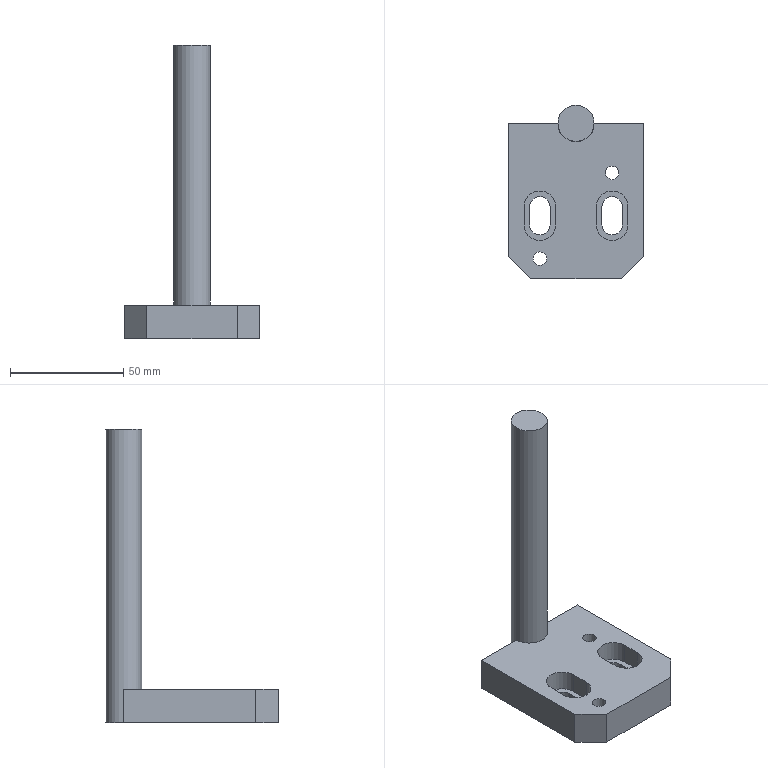Part | NX | features solid 2 | 1 solid | 31 faces | box 60 x 76.5 x 130 mm | volume 77518 mm3 | plane 20 | cylinder 11 | commonest cylinder face diameters 9 x4 14 x4 6 x2 16 x1
STEP:
#1=CARTESIAN_POINT('',(538.,-419.5,-140.));
#2=VERTEX_POINT('',#1);
#3=CARTESIAN_POINT('',(538.,-419.5,-125.));
#4=VERTEX_POINT('',#3);
#5=CARTESIAN_POINT('',(538.,-419.5,-140.));
#6=DIRECTION('',(0.,0.,1.));
#7=VECTOR('',#6,1000.);
#8=LINE('',#5,#7);
#9=EDGE_CURVE('',#2,#4,#8,.T.);
#10=ORIENTED_EDGE('',*,*,#9,.F.);
#11=CARTESIAN_POINT('',(522.,-419.5,-140.));
#12=VERTEX_POINT('',#11);
#13=CARTESIAN_POINT('',(530.,-419.5,-140.));
#14=DIRECTION('',(0.,0.,1.));
#15=DIRECTION('',(1.,0.,0.));
#16=AXIS2_PLACEMENT_3D('',#13,#14,#15);
#17=CIRCLE('',#16,8.);
#18=EDGE_CURVE('',#2,#12,#17,.T.);
#19=ORIENTED_EDGE('',*,*,#18,.T.);
#20=CARTESIAN_POINT('',(522.,-419.5,-125.));
#21=VERTEX_POINT('',#20);
#22=CARTESIAN_POINT('',(522.,-419.5,-140.));
#23=DIRECTION('',(0.,0.,1.));
#24=VECTOR('',#23,1000.);
#25=LINE('',#22,#24);
#26=EDGE_CURVE('',#21,#12,#25,.F.);
#27=ORIENTED_EDGE('',*,*,#26,.F.);
#28=CARTESIAN_POINT('',(530.,-419.5,-125.));
#29=DIRECTION('',(0.,0.,1.));
#30=DIRECTION('',(0.,1.,0.));
#31=AXIS2_PLACEMENT_3D('',#28,#29,#30);
#32=CIRCLE('',#31,8.);
#33=EDGE_CURVE('',#21,#4,#32,.T.);
#34=ORIENTED_EDGE('',*,*,#33,.T.);
#35=EDGE_LOOP('',(#10,#19,#27,#34));
#36=FACE_BOUND('',#35,.T.);
#37=CARTESIAN_POINT('',(522.,-419.5,-10.));
#38=VERTEX_POINT('',#37);
#39=CARTESIAN_POINT('',(530.,-419.5,-10.));
#40=DIRECTION('',(0.,0.,-1.));
#41=DIRECTION('',(-1.,0.,0.));
#42=AXIS2_PLACEMENT_3D('',#39,#40,#41);
#43=CIRCLE('',#42,8.);
#44=EDGE_CURVE('',#38,#38,#43,.F.);
#45=ORIENTED_EDGE('',*,*,#44,.F.);
#46=EDGE_LOOP('',(#45));
#47=FACE_BOUND('',#46,.T.);
#48=CARTESIAN_POINT('',(530.,-419.5,-140.));
#49=DIRECTION('',(0.,0.,1.));
#50=DIRECTION('',(0.,1.,0.));
#51=AXIS2_PLACEMENT_3D('',#48,#49,#50);
#52=CYLINDRICAL_SURFACE('',#51,8.);
#53=ADVANCED_FACE('',(#36,#47),#52,.T.);
#54=ORIENTED_EDGE('',*,*,#44,.T.);
#55=EDGE_LOOP('',(#54));
#56=FACE_BOUND('',#55,.T.);
#57=CARTESIAN_POINT('',(530.,-425.,-10.));
#58=DIRECTION('',(0.,0.,1.));
#59=DIRECTION('',(0.,1.,0.));
#60=AXIS2_PLACEMENT_3D('',#57,#58,#59);
#61=PLANE('',#60);
#62=ADVANCED_FACE('',(#56),#61,.T.);
#63=CARTESIAN_POINT('',(546.,-438.2,-125.));
#64=VERTEX_POINT('',#63);
#65=CARTESIAN_POINT('',(546.,-441.2,-125.));
#66=DIRECTION('',(0.,0.,1.));
#67=DIRECTION('',(0.,1.,0.));
#68=AXIS2_PLACEMENT_3D('',#65,#66,#67);
#69=CIRCLE('',#68,3.);
#70=EDGE_CURVE('',#64,#64,#69,.F.);
#71=ORIENTED_EDGE('',*,*,#70,.T.);
#72=EDGE_LOOP('',(#71));
#73=FACE_BOUND('',#72,.T.);
#74=CARTESIAN_POINT('',(539.,-456.2,-125.));
#75=VERTEX_POINT('',#74);
#76=CARTESIAN_POINT('',(553.,-456.2,-125.));
#77=VERTEX_POINT('',#76);
#78=CARTESIAN_POINT('',(546.,-456.2,-125.));
#79=DIRECTION('',(0.,0.,1.));
#80=DIRECTION('',(0.,1.,0.));
#81=AXIS2_PLACEMENT_3D('',#78,#79,#80);
#82=CIRCLE('',#81,7.);
#83=EDGE_CURVE('',#75,#77,#82,.F.);
#84=ORIENTED_EDGE('',*,*,#83,.T.);
#85=CARTESIAN_POINT('',(553.,-464.2,-125.));
#86=VERTEX_POINT('',#85);
#87=CARTESIAN_POINT('',(553.,-511.,-125.));
#88=DIRECTION('',(0.,-1.,0.));
#89=VECTOR('',#88,1000.);
#90=LINE('',#87,#89);
#91=EDGE_CURVE('',#77,#86,#90,.T.);
#92=ORIENTED_EDGE('',*,*,#91,.T.);
#93=CARTESIAN_POINT('',(539.,-464.2,-125.));
#94=VERTEX_POINT('',#93);
#95=CARTESIAN_POINT('',(546.,-464.2,-125.));
#96=DIRECTION('',(0.,0.,1.));
#97=DIRECTION('',(0.,1.,0.));
#98=AXIS2_PLACEMENT_3D('',#95,#96,#97);
#99=CIRCLE('',#98,7.);
#100=EDGE_CURVE('',#86,#94,#99,.F.);
#101=ORIENTED_EDGE('',*,*,#100,.T.);
#102=CARTESIAN_POINT('',(539.,-511.,-125.));
#103=DIRECTION('',(0.,-1.,0.));
#104=VECTOR('',#103,1000.);
#105=LINE('',#102,#104);
#106=EDGE_CURVE('',#75,#94,#105,.T.);
#107=ORIENTED_EDGE('',*,*,#106,.F.);
#108=EDGE_LOOP('',(#84,#92,#101,#107));
#109=FACE_BOUND('',#108,.T.);
#110=CARTESIAN_POINT('',(514.,-476.2,-125.));
#111=VERTEX_POINT('',#110);
#112=CARTESIAN_POINT('',(514.,-479.2,-125.));
#113=DIRECTION('',(0.,0.,1.));
#114=DIRECTION('',(0.,1.,0.));
#115=AXIS2_PLACEMENT_3D('',#112,#113,#114);
#116=CIRCLE('',#115,3.);
#117=EDGE_CURVE('',#111,#111,#116,.F.);
#118=ORIENTED_EDGE('',*,*,#117,.T.);
#119=EDGE_LOOP('',(#118));
#120=FACE_BOUND('',#119,.T.);
#121=CARTESIAN_POINT('',(507.,-456.2,-125.));
#122=VERTEX_POINT('',#121);
#123=CARTESIAN_POINT('',(507.,-464.2,-125.));
#124=VERTEX_POINT('',#123);
#125=CARTESIAN_POINT('',(507.,-456.2,-125.));
#126=DIRECTION('',(0.,-1.,0.));
#127=VECTOR('',#126,1000.);
#128=LINE('',#125,#127);
#129=EDGE_CURVE('',#122,#124,#128,.T.);
#130=ORIENTED_EDGE('',*,*,#129,.F.);
#131=CARTESIAN_POINT('',(521.,-456.2,-125.));
#132=VERTEX_POINT('',#131);
#133=CARTESIAN_POINT('',(514.,-456.2,-125.));
#134=DIRECTION('',(0.,0.,1.));
#135=DIRECTION('',(0.,1.,0.));
#136=AXIS2_PLACEMENT_3D('',#133,#134,#135);
#137=CIRCLE('',#136,7.);
#138=EDGE_CURVE('',#132,#122,#137,.T.);
#139=ORIENTED_EDGE('',*,*,#138,.F.);
#140=CARTESIAN_POINT('',(521.,-464.2,-125.));
#141=VERTEX_POINT('',#140);
#142=CARTESIAN_POINT('',(521.,-456.2,-125.));
#143=DIRECTION('',(0.,-1.,0.));
#144=VECTOR('',#143,1000.);
#145=LINE('',#142,#144);
#146=EDGE_CURVE('',#132,#141,#145,.T.);
#147=ORIENTED_EDGE('',*,*,#146,.T.);
#148=CARTESIAN_POINT('',(514.,-464.2,-125.));
#149=DIRECTION('',(0.,0.,1.));
#150=DIRECTION('',(0.,1.,0.));
#151=AXIS2_PLACEMENT_3D('',#148,#149,#150);
#152=CIRCLE('',#151,7.);
#153=EDGE_CURVE('',#124,#141,#152,.T.);
#154=ORIENTED_EDGE('',*,*,#153,.F.);
#155=EDGE_LOOP('',(#130,#139,#147,#154));
#156=FACE_BOUND('',#155,.T.);
#157=CARTESIAN_POINT('',(500.,-419.5,-125.));
#158=VERTEX_POINT('',#157);
#159=CARTESIAN_POINT('',(500.,-478.,-125.));
#160=VERTEX_POINT('',#159);
#161=CARTESIAN_POINT('',(500.,-431.,-125.));
#162=DIRECTION('',(0.,-1.,0.));
#163=VECTOR('',#162,1000.);
#164=LINE('',#161,#163);
#165=EDGE_CURVE('',#158,#160,#164,.T.);
#166=ORIENTED_EDGE('',*,*,#165,.T.);
#167=CARTESIAN_POINT('',(510.,-488.,-125.));
#168=VERTEX_POINT('',#167);
#169=CARTESIAN_POINT('',(531.5,-509.5,-125.));
#170=DIRECTION('',(-0.7071,0.7071,0.));
#171=VECTOR('',#170,1000.);
#172=LINE('',#169,#171);
#173=EDGE_CURVE('',#160,#168,#172,.F.);
#174=ORIENTED_EDGE('',*,*,#173,.T.);
#175=CARTESIAN_POINT('',(550.,-488.,-125.));
#176=VERTEX_POINT('',#175);
#177=CARTESIAN_POINT('',(530.,-488.,-125.));
#178=DIRECTION('',(-1.,0.,0.));
#179=VECTOR('',#178,1000.);
#180=LINE('',#177,#179);
#181=EDGE_CURVE('',#168,#176,#180,.F.);
#182=ORIENTED_EDGE('',*,*,#181,.T.);
#183=CARTESIAN_POINT('',(560.,-478.,-125.));
#184=VERTEX_POINT('',#183);
#185=CARTESIAN_POINT('',(528.5,-509.5,-125.));
#186=DIRECTION('',(0.7071,0.7071,0.));
#187=VECTOR('',#186,1000.);
#188=LINE('',#185,#187);
#189=EDGE_CURVE('',#176,#184,#188,.T.);
#190=ORIENTED_EDGE('',*,*,#189,.T.);
#191=CARTESIAN_POINT('',(560.,-419.5,-125.));
#192=VERTEX_POINT('',#191);
#193=CARTESIAN_POINT('',(560.,-431.,-125.));
#194=DIRECTION('',(0.,-1.,0.));
#195=VECTOR('',#194,1000.);
#196=LINE('',#193,#195);
#197=EDGE_CURVE('',#192,#184,#196,.T.);
#198=ORIENTED_EDGE('',*,*,#197,.F.);
#199=CARTESIAN_POINT('',(560.,-419.5,-125.));
#200=DIRECTION('',(-1.,0.,0.));
#201=VECTOR('',#200,1000.);
#202=LINE('',#199,#201);
#203=EDGE_CURVE('',#192,#4,#202,.T.);
#204=ORIENTED_EDGE('',*,*,#203,.T.);
#205=ORIENTED_EDGE('',*,*,#33,.F.);
#206=CARTESIAN_POINT('',(560.,-419.5,-125.));
#207=DIRECTION('',(-1.,0.,0.));
#208=VECTOR('',#207,1000.);
#209=LINE('',#206,#208);
#210=EDGE_CURVE('',#21,#158,#209,.T.);
#211=ORIENTED_EDGE('',*,*,#210,.T.);
#212=EDGE_LOOP('',(#166,#174,#182,#190,#198,#204,#205,#211));
#213=FACE_BOUND('',#212,.T.);
#214=CARTESIAN_POINT('',(530.,-511.,-125.));
#215=DIRECTION('',(0.,0.,1.));
#216=DIRECTION('',(0.,1.,0.));
#217=AXIS2_PLACEMENT_3D('',#214,#215,#216);
#218=PLANE('',#217);
#219=ADVANCED_FACE('',(#73,#109,#120,#156,#213),#218,.T.);
#220=CARTESIAN_POINT('',(546.,-438.2,-140.));
#221=VERTEX_POINT('',#220);
#222=CARTESIAN_POINT('',(546.,-441.2,-140.));
#223=DIRECTION('',(0.,0.,1.));
#224=DIRECTION('',(0.,1.,0.));
#225=AXIS2_PLACEMENT_3D('',#222,#223,#224);
#226=CIRCLE('',#225,3.);
#227=EDGE_CURVE('',#221,#221,#226,.T.);
#228=ORIENTED_EDGE('',*,*,#227,.T.);
#229=EDGE_LOOP('',(#228));
#230=FACE_BOUND('',#229,.T.);
#231=CARTESIAN_POINT('',(509.5,-464.2,-140.));
#232=VERTEX_POINT('',#231);
#233=CARTESIAN_POINT('',(518.5,-464.2,-140.));
#234=VERTEX_POINT('',#233);
#235=CARTESIAN_POINT('',(514.,-464.2,-140.));
#236=DIRECTION('',(0.,0.,1.));
#237=DIRECTION('',(0.,1.,0.));
#238=AXIS2_PLACEMENT_3D('',#235,#236,#237);
#239=CIRCLE('',#238,4.5);
#240=EDGE_CURVE('',#232,#234,#239,.T.);
#241=ORIENTED_EDGE('',*,*,#240,.T.);
#242=CARTESIAN_POINT('',(518.5,-456.2,-140.));
#243=VERTEX_POINT('',#242);
#244=CARTESIAN_POINT('',(518.5,-456.2,-140.));
#245=DIRECTION('',(0.,-1.,0.));
#246=VECTOR('',#245,1000.);
#247=LINE('',#244,#246);
#248=EDGE_CURVE('',#243,#234,#247,.T.);
#249=ORIENTED_EDGE('',*,*,#248,.F.);
#250=CARTESIAN_POINT('',(509.5,-456.2,-140.));
#251=VERTEX_POINT('',#250);
#252=CARTESIAN_POINT('',(514.,-456.2,-140.));
#253=DIRECTION('',(0.,0.,1.));
#254=DIRECTION('',(0.,1.,0.));
#255=AXIS2_PLACEMENT_3D('',#252,#253,#254);
#256=CIRCLE('',#255,4.5);
#257=EDGE_CURVE('',#243,#251,#256,.T.);
#258=ORIENTED_EDGE('',*,*,#257,.T.);
#259=CARTESIAN_POINT('',(509.5,-456.2,-140.));
#260=DIRECTION('',(0.,-1.,0.));
#261=VECTOR('',#260,1000.);
#262=LINE('',#259,#261);
#263=EDGE_CURVE('',#251,#232,#262,.T.);
#264=ORIENTED_EDGE('',*,*,#263,.T.);
#265=EDGE_LOOP('',(#241,#249,#258,#264));
#266=FACE_BOUND('',#265,.T.);
#267=CARTESIAN_POINT('',(514.,-476.2,-140.));
#268=VERTEX_POINT('',#267);
#269=CARTESIAN_POINT('',(514.,-479.2,-140.));
#270=DIRECTION('',(0.,0.,1.));
#271=DIRECTION('',(0.,1.,0.));
#272=AXIS2_PLACEMENT_3D('',#269,#270,#271);
#273=CIRCLE('',#272,3.);
#274=EDGE_CURVE('',#268,#268,#273,.T.);
#275=ORIENTED_EDGE('',*,*,#274,.T.);
#276=EDGE_LOOP('',(#275));
#277=FACE_BOUND('',#276,.T.);
#278=CARTESIAN_POINT('',(541.5,-464.2,-140.));
#279=VERTEX_POINT('',#278);
#280=CARTESIAN_POINT('',(550.5,-464.2,-140.));
#281=VERTEX_POINT('',#280);
#282=CARTESIAN_POINT('',(546.,-464.2,-140.));
#283=DIRECTION('',(0.,0.,1.));
#284=DIRECTION('',(0.,1.,0.));
#285=AXIS2_PLACEMENT_3D('',#282,#283,#284);
#286=CIRCLE('',#285,4.5);
#287=EDGE_CURVE('',#279,#281,#286,.T.);
#288=ORIENTED_EDGE('',*,*,#287,.T.);
#289=CARTESIAN_POINT('',(550.5,-456.2,-140.));
#290=VERTEX_POINT('',#289);
#291=CARTESIAN_POINT('',(550.5,-466.2,-140.));
#292=DIRECTION('',(0.,1.,0.));
#293=VECTOR('',#292,1000.);
#294=LINE('',#291,#293);
#295=EDGE_CURVE('',#281,#290,#294,.T.);
#296=ORIENTED_EDGE('',*,*,#295,.T.);
#297=CARTESIAN_POINT('',(541.5,-456.2,-140.));
#298=VERTEX_POINT('',#297);
#299=CARTESIAN_POINT('',(546.,-456.2,-140.));
#300=DIRECTION('',(0.,0.,1.));
#301=DIRECTION('',(0.,1.,0.));
#302=AXIS2_PLACEMENT_3D('',#299,#300,#301);
#303=CIRCLE('',#302,4.5);
#304=EDGE_CURVE('',#290,#298,#303,.T.);
#305=ORIENTED_EDGE('',*,*,#304,.T.);
#306=CARTESIAN_POINT('',(541.5,-466.2,-140.));
#307=DIRECTION('',(0.,1.,0.));
#308=VECTOR('',#307,1000.);
#309=LINE('',#306,#308);
#310=EDGE_CURVE('',#279,#298,#309,.T.);
#311=ORIENTED_EDGE('',*,*,#310,.F.);
#312=EDGE_LOOP('',(#288,#296,#305,#311));
#313=FACE_BOUND('',#312,.T.);
#314=CARTESIAN_POINT('',(550.,-488.,-140.));
#315=VERTEX_POINT('',#314);
#316=CARTESIAN_POINT('',(510.,-488.,-140.));
#317=VERTEX_POINT('',#316);
#318=CARTESIAN_POINT('',(570.,-488.,-140.));
#319=DIRECTION('',(1.,0.,0.));
#320=VECTOR('',#319,1000.);
#321=LINE('',#318,#320);
#322=EDGE_CURVE('',#315,#317,#321,.F.);
#323=ORIENTED_EDGE('',*,*,#322,.T.);
#324=CARTESIAN_POINT('',(500.,-478.,-140.));
#325=VERTEX_POINT('',#324);
#326=CARTESIAN_POINT('',(510.,-488.,-140.));
#327=DIRECTION('',(0.7071,-0.7071,0.));
#328=VECTOR('',#327,1000.);
#329=LINE('',#326,#328);
#330=EDGE_CURVE('',#317,#325,#329,.F.);
#331=ORIENTED_EDGE('',*,*,#330,.T.);
#332=CARTESIAN_POINT('',(500.,-419.5,-140.));
#333=VERTEX_POINT('',#332);
#334=CARTESIAN_POINT('',(500.,-431.,-140.));
#335=DIRECTION('',(0.,-1.,0.));
#336=VECTOR('',#335,1000.);
#337=LINE('',#334,#336);
#338=EDGE_CURVE('',#333,#325,#337,.T.);
#339=ORIENTED_EDGE('',*,*,#338,.F.);
#340=CARTESIAN_POINT('',(560.,-419.5,-140.));
#341=DIRECTION('',(-1.,0.,0.));
#342=VECTOR('',#341,1000.);
#343=LINE('',#340,#342);
#344=EDGE_CURVE('',#12,#333,#343,.T.);
#345=ORIENTED_EDGE('',*,*,#344,.F.);
#346=ORIENTED_EDGE('',*,*,#18,.F.);
#347=CARTESIAN_POINT('',(560.,-419.5,-140.));
#348=VERTEX_POINT('',#347);
#349=CARTESIAN_POINT('',(560.,-419.5,-140.));
#350=DIRECTION('',(-1.,0.,0.));
#351=VECTOR('',#350,1000.);
#352=LINE('',#349,#351);
#353=EDGE_CURVE('',#348,#2,#352,.T.);
#354=ORIENTED_EDGE('',*,*,#353,.F.);
#355=CARTESIAN_POINT('',(560.,-478.,-140.));
#356=VERTEX_POINT('',#355);
#357=CARTESIAN_POINT('',(560.,-431.,-140.));
#358=DIRECTION('',(0.,-1.,0.));
#359=VECTOR('',#358,1000.);
#360=LINE('',#357,#359);
#361=EDGE_CURVE('',#348,#356,#360,.T.);
#362=ORIENTED_EDGE('',*,*,#361,.T.);
#363=CARTESIAN_POINT('',(560.,-478.,-140.));
#364=DIRECTION('',(-0.7071,-0.7071,0.));
#365=VECTOR('',#364,1000.);
#366=LINE('',#363,#365);
#367=EDGE_CURVE('',#356,#315,#366,.T.);
#368=ORIENTED_EDGE('',*,*,#367,.T.);
#369=EDGE_LOOP('',(#323,#331,#339,#345,#346,#354,#362,#368));
#370=FACE_BOUND('',#369,.T.);
#371=CARTESIAN_POINT('',(530.,-511.,-140.));
#372=DIRECTION('',(0.,0.,1.));
#373=DIRECTION('',(0.,1.,0.));
#374=AXIS2_PLACEMENT_3D('',#371,#372,#373);
#375=PLANE('',#374);
#376=ADVANCED_FACE('',(#230,#266,#277,#313,#370),#375,.F.);
#377=ORIENTED_EDGE('',*,*,#197,.T.);
#378=CARTESIAN_POINT('',(560.,-478.,-125.));
#379=DIRECTION('',(0.,0.,-1.));
#380=VECTOR('',#379,1000.);
#381=LINE('',#378,#380);
#382=EDGE_CURVE('',#184,#356,#381,.T.);
#383=ORIENTED_EDGE('',*,*,#382,.T.);
#384=ORIENTED_EDGE('',*,*,#361,.F.);
#385=CARTESIAN_POINT('',(560.,-419.5,-125.));
#386=DIRECTION('',(0.,0.,-1.));
#387=VECTOR('',#386,1000.);
#388=LINE('',#385,#387);
#389=EDGE_CURVE('',#192,#348,#388,.T.);
#390=ORIENTED_EDGE('',*,*,#389,.F.);
#391=EDGE_LOOP('',(#377,#383,#384,#390));
#392=FACE_BOUND('',#391,.T.);
#393=CARTESIAN_POINT('',(560.,-431.,-125.));
#394=DIRECTION('',(1.,0.,0.));
#395=DIRECTION('',(0.,0.,-1.));
#396=AXIS2_PLACEMENT_3D('',#393,#394,#395);
#397=PLANE('',#396);
#398=ADVANCED_FACE('',(#392),#397,.T.);
#399=ORIENTED_EDGE('',*,*,#338,.T.);
#400=CARTESIAN_POINT('',(500.,-478.,-125.));
#401=DIRECTION('',(0.,0.,1.));
#402=VECTOR('',#401,1000.);
#403=LINE('',#400,#402);
#404=EDGE_CURVE('',#325,#160,#403,.T.);
#405=ORIENTED_EDGE('',*,*,#404,.T.);
#406=ORIENTED_EDGE('',*,*,#165,.F.);
#407=CARTESIAN_POINT('',(500.,-419.5,-125.));
#408=DIRECTION('',(0.,0.,-1.));
#409=VECTOR('',#408,1000.);
#410=LINE('',#407,#409);
#411=EDGE_CURVE('',#158,#333,#410,.T.);
#412=ORIENTED_EDGE('',*,*,#411,.T.);
#413=EDGE_LOOP('',(#399,#405,#406,#412));
#414=FACE_BOUND('',#413,.T.);
#415=CARTESIAN_POINT('',(500.,-431.,-125.));
#416=DIRECTION('',(1.,0.,0.));
#417=DIRECTION('',(0.,1.,0.));
#418=AXIS2_PLACEMENT_3D('',#415,#416,#417);
#419=PLANE('',#418);
#420=ADVANCED_FACE('',(#414),#419,.F.);
#421=ORIENTED_EDGE('',*,*,#353,.T.);
#422=ORIENTED_EDGE('',*,*,#9,.T.);
#423=ORIENTED_EDGE('',*,*,#203,.F.);
#424=ORIENTED_EDGE('',*,*,#389,.T.);
#425=EDGE_LOOP('',(#421,#422,#423,#424));
#426=FACE_BOUND('',#425,.T.);
#427=CARTESIAN_POINT('',(560.,-419.5,-125.));
#428=DIRECTION('',(0.,-1.,0.));
#429=DIRECTION('',(0.,0.,1.));
#430=AXIS2_PLACEMENT_3D('',#427,#428,#429);
#431=PLANE('',#430);
#432=ADVANCED_FACE('',(#426),#431,.F.);
#433=CARTESIAN_POINT('',(518.5,-456.2,-134.));
#434=VERTEX_POINT('',#433);
#435=CARTESIAN_POINT('',(518.5,-464.2,-134.));
#436=VERTEX_POINT('',#435);
#437=CARTESIAN_POINT('',(518.5,-456.2,-134.));
#438=DIRECTION('',(0.,-1.,0.));
#439=VECTOR('',#438,1000.);
#440=LINE('',#437,#439);
#441=EDGE_CURVE('',#434,#436,#440,.T.);
#442=ORIENTED_EDGE('',*,*,#441,.F.);
#443=CARTESIAN_POINT('',(518.5,-456.2,-124.));
#444=DIRECTION('',(0.,0.,-1.));
#445=VECTOR('',#444,1000.);
#446=LINE('',#443,#445);
#447=EDGE_CURVE('',#434,#243,#446,.T.);
#448=ORIENTED_EDGE('',*,*,#447,.T.);
#449=ORIENTED_EDGE('',*,*,#248,.T.);
#450=CARTESIAN_POINT('',(518.5,-464.2,-124.));
#451=DIRECTION('',(0.,0.,-1.));
#452=VECTOR('',#451,1000.);
#453=LINE('',#450,#452);
#454=EDGE_CURVE('',#436,#234,#453,.T.);
#455=ORIENTED_EDGE('',*,*,#454,.F.);
#456=EDGE_LOOP('',(#442,#448,#449,#455));
#457=FACE_BOUND('',#456,.T.);
#458=CARTESIAN_POINT('',(518.5,-456.2,-124.));
#459=DIRECTION('',(1.,0.,0.));
#460=DIRECTION('',(0.,0.,-1.));
#461=AXIS2_PLACEMENT_3D('',#458,#459,#460);
#462=PLANE('',#461);
#463=ADVANCED_FACE('',(#457),#462,.F.);
#464=ORIENTED_EDGE('',*,*,#447,.F.);
#465=CARTESIAN_POINT('',(509.5,-456.2,-134.));
#466=VERTEX_POINT('',#465);
#467=CARTESIAN_POINT('',(514.,-456.2,-134.));
#468=DIRECTION('',(0.,0.,1.));
#469=DIRECTION('',(0.,1.,0.));
#470=AXIS2_PLACEMENT_3D('',#467,#468,#469);
#471=CIRCLE('',#470,4.5);
#472=EDGE_CURVE('',#434,#466,#471,.T.);
#473=ORIENTED_EDGE('',*,*,#472,.T.);
#474=CARTESIAN_POINT('',(509.5,-456.2,-124.));
#475=DIRECTION('',(0.,0.,-1.));
#476=VECTOR('',#475,1000.);
#477=LINE('',#474,#476);
#478=EDGE_CURVE('',#466,#251,#477,.T.);
#479=ORIENTED_EDGE('',*,*,#478,.T.);
#480=ORIENTED_EDGE('',*,*,#257,.F.);
#481=EDGE_LOOP('',(#464,#473,#479,#480));
#482=FACE_BOUND('',#481,.T.);
#483=CARTESIAN_POINT('',(514.,-456.2,-124.));
#484=DIRECTION('',(0.,0.,-1.));
#485=DIRECTION('',(0.,-1.,0.));
#486=AXIS2_PLACEMENT_3D('',#483,#484,#485);
#487=CYLINDRICAL_SURFACE('',#486,4.5);
#488=ADVANCED_FACE('',(#482),#487,.F.);
#489=ORIENTED_EDGE('',*,*,#478,.F.);
#490=CARTESIAN_POINT('',(509.5,-464.2,-134.));
#491=VERTEX_POINT('',#490);
#492=CARTESIAN_POINT('',(509.5,-456.2,-134.));
#493=DIRECTION('',(0.,-1.,0.));
#494=VECTOR('',#493,1000.);
#495=LINE('',#492,#494);
#496=EDGE_CURVE('',#466,#491,#495,.T.);
#497=ORIENTED_EDGE('',*,*,#496,.T.);
#498=CARTESIAN_POINT('',(509.5,-464.2,-124.));
#499=DIRECTION('',(0.,0.,-1.));
#500=VECTOR('',#499,1000.);
#501=LINE('',#498,#500);
#502=EDGE_CURVE('',#491,#232,#501,.T.);
#503=ORIENTED_EDGE('',*,*,#502,.T.);
#504=ORIENTED_EDGE('',*,*,#263,.F.);
#505=EDGE_LOOP('',(#489,#497,#503,#504));
#506=FACE_BOUND('',#505,.T.);
#507=CARTESIAN_POINT('',(509.5,-456.2,-124.));
#508=DIRECTION('',(1.,0.,0.));
#509=DIRECTION('',(0.,0.,-1.));
#510=AXIS2_PLACEMENT_3D('',#507,#508,#509);
#511=PLANE('',#510);
#512=ADVANCED_FACE('',(#506),#511,.T.);
#513=ORIENTED_EDGE('',*,*,#502,.F.);
#514=CARTESIAN_POINT('',(514.,-464.2,-134.));
#515=DIRECTION('',(0.,0.,1.));
#516=DIRECTION('',(0.,1.,0.));
#517=AXIS2_PLACEMENT_3D('',#514,#515,#516);
#518=CIRCLE('',#517,4.5);
#519=EDGE_CURVE('',#491,#436,#518,.T.);
#520=ORIENTED_EDGE('',*,*,#519,.T.);
#521=ORIENTED_EDGE('',*,*,#454,.T.);
#522=ORIENTED_EDGE('',*,*,#240,.F.);
#523=EDGE_LOOP('',(#513,#520,#521,#522));
#524=FACE_BOUND('',#523,.T.);
#525=CARTESIAN_POINT('',(514.,-464.2,-124.));
#526=DIRECTION('',(0.,0.,-1.));
#527=DIRECTION('',(0.,-1.,0.));
#528=AXIS2_PLACEMENT_3D('',#525,#526,#527);
#529=CYLINDRICAL_SURFACE('',#528,4.5);
#530=ADVANCED_FACE('',(#524),#529,.F.);
#531=ORIENTED_EDGE('',*,*,#210,.F.);
#532=ORIENTED_EDGE('',*,*,#26,.T.);
#533=ORIENTED_EDGE('',*,*,#344,.T.);
#534=ORIENTED_EDGE('',*,*,#411,.F.);
#535=EDGE_LOOP('',(#531,#532,#533,#534));
#536=FACE_BOUND('',#535,.T.);
#537=CARTESIAN_POINT('',(560.,-419.5,-125.));
#538=DIRECTION('',(0.,-1.,0.));
#539=DIRECTION('',(0.,0.,1.));
#540=AXIS2_PLACEMENT_3D('',#537,#538,#539);
#541=PLANE('',#540);
#542=ADVANCED_FACE('',(#536),#541,.F.);
#543=CARTESIAN_POINT('',(553.,-456.2,-134.));
#544=VERTEX_POINT('',#543);
#545=CARTESIAN_POINT('',(553.,-456.2,-124.));
#546=DIRECTION('',(0.,0.,-1.));
#547=VECTOR('',#546,1000.);
#548=LINE('',#545,#547);
#549=EDGE_CURVE('',#77,#544,#548,.T.);
#550=ORIENTED_EDGE('',*,*,#549,.T.);
#551=CARTESIAN_POINT('',(553.,-464.2,-134.));
#552=VERTEX_POINT('',#551);
#553=CARTESIAN_POINT('',(553.,-466.2,-134.));
#554=DIRECTION('',(0.,1.,0.));
#555=VECTOR('',#554,1000.);
#556=LINE('',#553,#555);
#557=EDGE_CURVE('',#552,#544,#556,.T.);
#558=ORIENTED_EDGE('',*,*,#557,.F.);
#559=CARTESIAN_POINT('',(553.,-464.2,-124.));
#560=DIRECTION('',(0.,0.,-1.));
#561=VECTOR('',#560,1000.);
#562=LINE('',#559,#561);
#563=EDGE_CURVE('',#86,#552,#562,.T.);
#564=ORIENTED_EDGE('',*,*,#563,.F.);
#565=ORIENTED_EDGE('',*,*,#91,.F.);
#566=EDGE_LOOP('',(#550,#558,#564,#565));
#567=FACE_BOUND('',#566,.T.);
#568=CARTESIAN_POINT('',(553.,-466.2,-124.));
#569=DIRECTION('',(-1.,0.,0.));
#570=DIRECTION('',(0.,0.,1.));
#571=AXIS2_PLACEMENT_3D('',#568,#569,#570);
#572=PLANE('',#571);
#573=ADVANCED_FACE('',(#567),#572,.T.);
#574=CARTESIAN_POINT('',(539.,-456.2,-134.));
#575=VERTEX_POINT('',#574);
#576=CARTESIAN_POINT('',(539.,-456.2,-124.));
#577=DIRECTION('',(0.,0.,-1.));
#578=VECTOR('',#577,1000.);
#579=LINE('',#576,#578);
#580=EDGE_CURVE('',#75,#575,#579,.T.);
#581=ORIENTED_EDGE('',*,*,#580,.T.);
#582=CARTESIAN_POINT('',(546.,-456.2,-134.));
#583=DIRECTION('',(0.,0.,1.));
#584=DIRECTION('',(0.,1.,0.));
#585=AXIS2_PLACEMENT_3D('',#582,#583,#584);
#586=CIRCLE('',#585,7.);
#587=EDGE_CURVE('',#544,#575,#586,.T.);
#588=ORIENTED_EDGE('',*,*,#587,.F.);
#589=ORIENTED_EDGE('',*,*,#549,.F.);
#590=ORIENTED_EDGE('',*,*,#83,.F.);
#591=EDGE_LOOP('',(#581,#588,#589,#590));
#592=FACE_BOUND('',#591,.T.);
#593=CARTESIAN_POINT('',(546.,-456.2,-124.));
#594=DIRECTION('',(0.,0.,-1.));
#595=DIRECTION('',(0.,-1.,0.));
#596=AXIS2_PLACEMENT_3D('',#593,#594,#595);
#597=CYLINDRICAL_SURFACE('',#596,7.);
#598=ADVANCED_FACE('',(#592),#597,.F.);
#599=ORIENTED_EDGE('',*,*,#106,.T.);
#600=CARTESIAN_POINT('',(539.,-464.2,-134.));
#601=VERTEX_POINT('',#600);
#602=CARTESIAN_POINT('',(539.,-464.2,-124.));
#603=DIRECTION('',(0.,0.,-1.));
#604=VECTOR('',#603,1000.);
#605=LINE('',#602,#604);
#606=EDGE_CURVE('',#94,#601,#605,.T.);
#607=ORIENTED_EDGE('',*,*,#606,.T.);
#608=CARTESIAN_POINT('',(539.,-466.2,-134.));
#609=DIRECTION('',(0.,1.,0.));
#610=VECTOR('',#609,1000.);
#611=LINE('',#608,#610);
#612=EDGE_CURVE('',#601,#575,#611,.T.);
#613=ORIENTED_EDGE('',*,*,#612,.T.);
#614=ORIENTED_EDGE('',*,*,#580,.F.);
#615=EDGE_LOOP('',(#599,#607,#613,#614));
#616=FACE_BOUND('',#615,.T.);
#617=CARTESIAN_POINT('',(539.,-466.2,-124.));
#618=DIRECTION('',(-1.,0.,0.));
#619=DIRECTION('',(0.,0.,1.));
#620=AXIS2_PLACEMENT_3D('',#617,#618,#619);
#621=PLANE('',#620);
#622=ADVANCED_FACE('',(#616),#621,.F.);
#623=ORIENTED_EDGE('',*,*,#563,.T.);
#624=CARTESIAN_POINT('',(546.,-464.2,-134.));
#625=DIRECTION('',(0.,0.,1.));
#626=DIRECTION('',(0.,1.,0.));
#627=AXIS2_PLACEMENT_3D('',#624,#625,#626);
#628=CIRCLE('',#627,7.);
#629=EDGE_CURVE('',#601,#552,#628,.T.);
#630=ORIENTED_EDGE('',*,*,#629,.F.);
#631=ORIENTED_EDGE('',*,*,#606,.F.);
#632=ORIENTED_EDGE('',*,*,#100,.F.);
#633=EDGE_LOOP('',(#623,#630,#631,#632));
#634=FACE_BOUND('',#633,.T.);
#635=CARTESIAN_POINT('',(546.,-464.2,-124.));
#636=DIRECTION('',(0.,0.,-1.));
#637=DIRECTION('',(0.,-1.,0.));
#638=AXIS2_PLACEMENT_3D('',#635,#636,#637);
#639=CYLINDRICAL_SURFACE('',#638,7.);
#640=ADVANCED_FACE('',(#634),#639,.F.);
#641=CARTESIAN_POINT('',(550.5,-464.2,-134.));
#642=VERTEX_POINT('',#641);
#643=CARTESIAN_POINT('',(550.5,-456.2,-134.));
#644=VERTEX_POINT('',#643);
#645=CARTESIAN_POINT('',(550.5,-466.2,-134.));
#646=DIRECTION('',(0.,1.,0.));
#647=VECTOR('',#646,1000.);
#648=LINE('',#645,#647);
#649=EDGE_CURVE('',#642,#644,#648,.T.);
#650=ORIENTED_EDGE('',*,*,#649,.F.);
#651=CARTESIAN_POINT('',(541.5,-464.2,-134.));
#652=VERTEX_POINT('',#651);
#653=CARTESIAN_POINT('',(546.,-464.2,-134.));
#654=DIRECTION('',(0.,0.,1.));
#655=DIRECTION('',(0.,1.,0.));
#656=AXIS2_PLACEMENT_3D('',#653,#654,#655);
#657=CIRCLE('',#656,4.5);
#658=EDGE_CURVE('',#652,#642,#657,.T.);
#659=ORIENTED_EDGE('',*,*,#658,.F.);
#660=CARTESIAN_POINT('',(541.5,-456.2,-134.));
#661=VERTEX_POINT('',#660);
#662=CARTESIAN_POINT('',(541.5,-466.2,-134.));
#663=DIRECTION('',(0.,1.,0.));
#664=VECTOR('',#663,1000.);
#665=LINE('',#662,#664);
#666=EDGE_CURVE('',#652,#661,#665,.T.);
#667=ORIENTED_EDGE('',*,*,#666,.T.);
#668=CARTESIAN_POINT('',(546.,-456.2,-134.));
#669=DIRECTION('',(0.,0.,1.));
#670=DIRECTION('',(0.,1.,0.));
#671=AXIS2_PLACEMENT_3D('',#668,#669,#670);
#672=CIRCLE('',#671,4.5);
#673=EDGE_CURVE('',#644,#661,#672,.T.);
#674=ORIENTED_EDGE('',*,*,#673,.F.);
#675=EDGE_LOOP('',(#650,#659,#667,#674));
#676=FACE_BOUND('',#675,.T.);
#677=ORIENTED_EDGE('',*,*,#557,.T.);
#678=ORIENTED_EDGE('',*,*,#587,.T.);
#679=ORIENTED_EDGE('',*,*,#612,.F.);
#680=ORIENTED_EDGE('',*,*,#629,.T.);
#681=EDGE_LOOP('',(#677,#678,#679,#680));
#682=FACE_BOUND('',#681,.T.);
#683=CARTESIAN_POINT('',(546.,-466.2,-134.));
#684=DIRECTION('',(0.,0.,1.));
#685=DIRECTION('',(0.,1.,0.));
#686=AXIS2_PLACEMENT_3D('',#683,#684,#685);
#687=PLANE('',#686);
#688=ADVANCED_FACE('',(#676,#682),#687,.T.);
#689=ORIENTED_EDGE('',*,*,#117,.F.);
#690=EDGE_LOOP('',(#689));
#691=FACE_BOUND('',#690,.T.);
#692=ORIENTED_EDGE('',*,*,#274,.F.);
#693=EDGE_LOOP('',(#692));
#694=FACE_BOUND('',#693,.T.);
#695=CARTESIAN_POINT('',(514.,-479.2,-124.));
#696=DIRECTION('',(0.,0.,-1.));
#697=DIRECTION('',(0.,-1.,0.));
#698=AXIS2_PLACEMENT_3D('',#695,#696,#697);
#699=CYLINDRICAL_SURFACE('',#698,3.);
#700=ADVANCED_FACE('',(#691,#694),#699,.F.);
#701=ORIENTED_EDGE('',*,*,#70,.F.);
#702=EDGE_LOOP('',(#701));
#703=FACE_BOUND('',#702,.T.);
#704=ORIENTED_EDGE('',*,*,#227,.F.);
#705=EDGE_LOOP('',(#704));
#706=FACE_BOUND('',#705,.T.);
#707=CARTESIAN_POINT('',(546.,-441.2,-124.));
#708=DIRECTION('',(0.,0.,-1.));
#709=DIRECTION('',(0.,-1.,0.));
#710=AXIS2_PLACEMENT_3D('',#707,#708,#709);
#711=CYLINDRICAL_SURFACE('',#710,3.);
#712=ADVANCED_FACE('',(#703,#706),#711,.F.);
#713=CARTESIAN_POINT('',(507.,-456.2,-134.));
#714=VERTEX_POINT('',#713);
#715=CARTESIAN_POINT('',(507.,-464.2,-134.));
#716=VERTEX_POINT('',#715);
#717=CARTESIAN_POINT('',(507.,-456.2,-134.));
#718=DIRECTION('',(0.,-1.,0.));
#719=VECTOR('',#718,1000.);
#720=LINE('',#717,#719);
#721=EDGE_CURVE('',#714,#716,#720,.T.);
#722=ORIENTED_EDGE('',*,*,#721,.T.);
#723=CARTESIAN_POINT('',(521.,-464.2,-134.));
#724=VERTEX_POINT('',#723);
#725=CARTESIAN_POINT('',(514.,-464.2,-134.));
#726=DIRECTION('',(0.,0.,1.));
#727=DIRECTION('',(0.,1.,0.));
#728=AXIS2_PLACEMENT_3D('',#725,#726,#727);
#729=CIRCLE('',#728,7.);
#730=EDGE_CURVE('',#716,#724,#729,.T.);
#731=ORIENTED_EDGE('',*,*,#730,.T.);
#732=CARTESIAN_POINT('',(521.,-456.2,-134.));
#733=VERTEX_POINT('',#732);
#734=CARTESIAN_POINT('',(521.,-456.2,-134.));
#735=DIRECTION('',(0.,-1.,0.));
#736=VECTOR('',#735,1000.);
#737=LINE('',#734,#736);
#738=EDGE_CURVE('',#733,#724,#737,.T.);
#739=ORIENTED_EDGE('',*,*,#738,.F.);
#740=CARTESIAN_POINT('',(514.,-456.2,-134.));
#741=DIRECTION('',(0.,0.,1.));
#742=DIRECTION('',(0.,1.,0.));
#743=AXIS2_PLACEMENT_3D('',#740,#741,#742);
#744=CIRCLE('',#743,7.);
#745=EDGE_CURVE('',#733,#714,#744,.T.);
#746=ORIENTED_EDGE('',*,*,#745,.T.);
#747=EDGE_LOOP('',(#722,#731,#739,#746));
#748=FACE_BOUND('',#747,.T.);
#749=ORIENTED_EDGE('',*,*,#441,.T.);
#750=ORIENTED_EDGE('',*,*,#519,.F.);
#751=ORIENTED_EDGE('',*,*,#496,.F.);
#752=ORIENTED_EDGE('',*,*,#472,.F.);
#753=EDGE_LOOP('',(#749,#750,#751,#752));
#754=FACE_BOUND('',#753,.T.);
#755=CARTESIAN_POINT('',(514.,-466.2,-134.));
#756=DIRECTION('',(0.,0.,1.));
#757=DIRECTION('',(0.,1.,0.));
#758=AXIS2_PLACEMENT_3D('',#755,#756,#757);
#759=PLANE('',#758);
#760=ADVANCED_FACE('',(#748,#754),#759,.T.);
#761=ORIENTED_EDGE('',*,*,#129,.T.);
#762=CARTESIAN_POINT('',(507.,-464.2,-134.));
#763=DIRECTION('',(0.,0.,1.));
#764=VECTOR('',#763,1000.);
#765=LINE('',#762,#764);
#766=EDGE_CURVE('',#716,#124,#765,.T.);
#767=ORIENTED_EDGE('',*,*,#766,.F.);
#768=ORIENTED_EDGE('',*,*,#721,.F.);
#769=CARTESIAN_POINT('',(507.,-456.2,-134.));
#770=DIRECTION('',(0.,0.,1.));
#771=VECTOR('',#770,1000.);
#772=LINE('',#769,#771);
#773=EDGE_CURVE('',#714,#122,#772,.T.);
#774=ORIENTED_EDGE('',*,*,#773,.T.);
#775=EDGE_LOOP('',(#761,#767,#768,#774));
#776=FACE_BOUND('',#775,.T.);
#777=CARTESIAN_POINT('',(507.,-456.2,-134.));
#778=DIRECTION('',(-1.,0.,0.));
#779=DIRECTION('',(0.,0.,1.));
#780=AXIS2_PLACEMENT_3D('',#777,#778,#779);
#781=PLANE('',#780);
#782=ADVANCED_FACE('',(#776),#781,.F.);
#783=ORIENTED_EDGE('',*,*,#153,.T.);
#784=CARTESIAN_POINT('',(521.,-464.2,-134.));
#785=DIRECTION('',(0.,0.,1.));
#786=VECTOR('',#785,1000.);
#787=LINE('',#784,#786);
#788=EDGE_CURVE('',#724,#141,#787,.T.);
#789=ORIENTED_EDGE('',*,*,#788,.F.);
#790=ORIENTED_EDGE('',*,*,#730,.F.);
#791=ORIENTED_EDGE('',*,*,#766,.T.);
#792=EDGE_LOOP('',(#783,#789,#790,#791));
#793=FACE_BOUND('',#792,.T.);
#794=CARTESIAN_POINT('',(514.,-464.2,-134.));
#795=DIRECTION('',(0.,0.,1.));
#796=DIRECTION('',(0.,1.,0.));
#797=AXIS2_PLACEMENT_3D('',#794,#795,#796);
#798=CYLINDRICAL_SURFACE('',#797,7.);
#799=ADVANCED_FACE('',(#793),#798,.F.);
#800=ORIENTED_EDGE('',*,*,#146,.F.);
#801=CARTESIAN_POINT('',(521.,-456.2,-134.));
#802=DIRECTION('',(0.,0.,1.));
#803=VECTOR('',#802,1000.);
#804=LINE('',#801,#803);
#805=EDGE_CURVE('',#733,#132,#804,.T.);
#806=ORIENTED_EDGE('',*,*,#805,.F.);
#807=ORIENTED_EDGE('',*,*,#738,.T.);
#808=ORIENTED_EDGE('',*,*,#788,.T.);
#809=EDGE_LOOP('',(#800,#806,#807,#808));
#810=FACE_BOUND('',#809,.T.);
#811=CARTESIAN_POINT('',(521.,-456.2,-134.));
#812=DIRECTION('',(-1.,0.,0.));
#813=DIRECTION('',(0.,0.,1.));
#814=AXIS2_PLACEMENT_3D('',#811,#812,#813);
#815=PLANE('',#814);
#816=ADVANCED_FACE('',(#810),#815,.T.);
#817=ORIENTED_EDGE('',*,*,#138,.T.);
#818=ORIENTED_EDGE('',*,*,#773,.F.);
#819=ORIENTED_EDGE('',*,*,#745,.F.);
#820=ORIENTED_EDGE('',*,*,#805,.T.);
#821=EDGE_LOOP('',(#817,#818,#819,#820));
#822=FACE_BOUND('',#821,.T.);
#823=CARTESIAN_POINT('',(514.,-456.2,-134.));
#824=DIRECTION('',(0.,0.,1.));
#825=DIRECTION('',(0.,1.,0.));
#826=AXIS2_PLACEMENT_3D('',#823,#824,#825);
#827=CYLINDRICAL_SURFACE('',#826,7.);
#828=ADVANCED_FACE('',(#822),#827,.F.);
#829=ORIENTED_EDGE('',*,*,#649,.T.);
#830=CARTESIAN_POINT('',(550.5,-456.2,-140.));
#831=DIRECTION('',(0.,0.,1.));
#832=VECTOR('',#831,1000.);
#833=LINE('',#830,#832);
#834=EDGE_CURVE('',#290,#644,#833,.T.);
#835=ORIENTED_EDGE('',*,*,#834,.F.);
#836=ORIENTED_EDGE('',*,*,#295,.F.);
#837=CARTESIAN_POINT('',(550.5,-464.2,-140.));
#838=DIRECTION('',(0.,0.,1.));
#839=VECTOR('',#838,1000.);
#840=LINE('',#837,#839);
#841=EDGE_CURVE('',#281,#642,#840,.T.);
#842=ORIENTED_EDGE('',*,*,#841,.T.);
#843=EDGE_LOOP('',(#829,#835,#836,#842));
#844=FACE_BOUND('',#843,.T.);
#845=CARTESIAN_POINT('',(550.5,-466.2,-140.));
#846=DIRECTION('',(1.,0.,0.));
#847=DIRECTION('',(0.,0.,-1.));
#848=AXIS2_PLACEMENT_3D('',#845,#846,#847);
#849=PLANE('',#848);
#850=ADVANCED_FACE('',(#844),#849,.F.);
#851=ORIENTED_EDGE('',*,*,#673,.T.);
#852=CARTESIAN_POINT('',(541.5,-456.2,-140.));
#853=DIRECTION('',(0.,0.,1.));
#854=VECTOR('',#853,1000.);
#855=LINE('',#852,#854);
#856=EDGE_CURVE('',#298,#661,#855,.T.);
#857=ORIENTED_EDGE('',*,*,#856,.F.);
#858=ORIENTED_EDGE('',*,*,#304,.F.);
#859=ORIENTED_EDGE('',*,*,#834,.T.);
#860=EDGE_LOOP('',(#851,#857,#858,#859));
#861=FACE_BOUND('',#860,.T.);
#862=CARTESIAN_POINT('',(546.,-456.2,-140.));
#863=DIRECTION('',(0.,0.,1.));
#864=DIRECTION('',(0.,1.,0.));
#865=AXIS2_PLACEMENT_3D('',#862,#863,#864);
#866=CYLINDRICAL_SURFACE('',#865,4.5);
#867=ADVANCED_FACE('',(#861),#866,.F.);
#868=ORIENTED_EDGE('',*,*,#666,.F.);
#869=CARTESIAN_POINT('',(541.5,-464.2,-140.));
#870=DIRECTION('',(0.,0.,1.));
#871=VECTOR('',#870,1000.);
#872=LINE('',#869,#871);
#873=EDGE_CURVE('',#279,#652,#872,.T.);
#874=ORIENTED_EDGE('',*,*,#873,.F.);
#875=ORIENTED_EDGE('',*,*,#310,.T.);
#876=ORIENTED_EDGE('',*,*,#856,.T.);
#877=EDGE_LOOP('',(#868,#874,#875,#876));
#878=FACE_BOUND('',#877,.T.);
#879=CARTESIAN_POINT('',(541.5,-466.2,-140.));
#880=DIRECTION('',(1.,0.,0.));
#881=DIRECTION('',(0.,0.,-1.));
#882=AXIS2_PLACEMENT_3D('',#879,#880,#881);
#883=PLANE('',#882);
#884=ADVANCED_FACE('',(#878),#883,.T.);
#885=ORIENTED_EDGE('',*,*,#658,.T.);
#886=ORIENTED_EDGE('',*,*,#841,.F.);
#887=ORIENTED_EDGE('',*,*,#287,.F.);
#888=ORIENTED_EDGE('',*,*,#873,.T.);
#889=EDGE_LOOP('',(#885,#886,#887,#888));
#890=FACE_BOUND('',#889,.T.);
#891=CARTESIAN_POINT('',(546.,-464.2,-140.));
#892=DIRECTION('',(0.,0.,1.));
#893=DIRECTION('',(0.,1.,0.));
#894=AXIS2_PLACEMENT_3D('',#891,#892,#893);
#895=CYLINDRICAL_SURFACE('',#894,4.5);
#896=ADVANCED_FACE('',(#890),#895,.F.);
#897=ORIENTED_EDGE('',*,*,#181,.F.);
#898=CARTESIAN_POINT('',(510.,-488.,-140.));
#899=DIRECTION('',(0.,0.,1.));
#900=VECTOR('',#899,1000.);
#901=LINE('',#898,#900);
#902=EDGE_CURVE('',#168,#317,#901,.F.);
#903=ORIENTED_EDGE('',*,*,#902,.T.);
#904=ORIENTED_EDGE('',*,*,#322,.F.);
#905=CARTESIAN_POINT('',(550.,-488.,-140.));
#906=DIRECTION('',(0.,0.,-1.));
#907=VECTOR('',#906,1000.);
#908=LINE('',#905,#907);
#909=EDGE_CURVE('',#315,#176,#908,.F.);
#910=ORIENTED_EDGE('',*,*,#909,.T.);
#911=EDGE_LOOP('',(#897,#903,#904,#910));
#912=FACE_BOUND('',#911,.T.);
#913=CARTESIAN_POINT('',(570.,-488.,-140.));
#914=DIRECTION('',(0.,1.,0.));
#915=DIRECTION('',(-1.,0.,0.));
#916=AXIS2_PLACEMENT_3D('',#913,#914,#915);
#917=PLANE('',#916);
#918=ADVANCED_FACE('',(#912),#917,.F.);
#919=ORIENTED_EDGE('',*,*,#189,.F.);
#920=ORIENTED_EDGE('',*,*,#909,.F.);
#921=ORIENTED_EDGE('',*,*,#367,.F.);
#922=ORIENTED_EDGE('',*,*,#382,.F.);
#923=EDGE_LOOP('',(#919,#920,#921,#922));
#924=FACE_BOUND('',#923,.T.);
#925=CARTESIAN_POINT('',(560.,-478.,-125.));
#926=DIRECTION('',(0.7071,-0.7071,0.));
#927=DIRECTION('',(0.7071,0.7071,0.));
#928=AXIS2_PLACEMENT_3D('',#925,#926,#927);
#929=PLANE('',#928);
#930=ADVANCED_FACE('',(#924),#929,.T.);
#931=ORIENTED_EDGE('',*,*,#173,.F.);
#932=ORIENTED_EDGE('',*,*,#404,.F.);
#933=ORIENTED_EDGE('',*,*,#330,.F.);
#934=ORIENTED_EDGE('',*,*,#902,.F.);
#935=EDGE_LOOP('',(#931,#932,#933,#934));
#936=FACE_BOUND('',#935,.T.);
#937=CARTESIAN_POINT('',(510.,-488.,-140.));
#938=DIRECTION('',(0.7071,0.7071,0.));
#939=DIRECTION('',(-0.7071,0.7071,0.));
#940=AXIS2_PLACEMENT_3D('',#937,#938,#939);
#941=PLANE('',#940);
#942=ADVANCED_FACE('',(#936),#941,.F.);
#943=CLOSED_SHELL('',(#53,#62,#219,#376,#398,#420,#432,#463,#488,#512,#530,#542,#573,#598,#622,#640,#688,#700,#712,#760,#782,#799,#816,#828,#850,#867,#884,#896,#918,#930,#942));
#944=MANIFOLD_SOLID_BREP('',#943);
#945=(LENGTH_UNIT()NAMED_UNIT(*)SI_UNIT(.MILLI.,.METRE.));
#946=UNCERTAINTY_MEASURE_WITH_UNIT(LENGTH_MEASURE(0.00001),#945,'','');
#947=(NAMED_UNIT(*)PLANE_ANGLE_UNIT()SI_UNIT($,.RADIAN.));
#948=(NAMED_UNIT(*)SI_UNIT($,.STERADIAN.)SOLID_ANGLE_UNIT());
#949=(GEOMETRIC_REPRESENTATION_CONTEXT(3)GLOBAL_UNCERTAINTY_ASSIGNED_CONTEXT((#946))GLOBAL_UNIT_ASSIGNED_CONTEXT((#945,#947,#948))REPRESENTATION_CONTEXT('',''));
#950=ADVANCED_BREP_SHAPE_REPRESENTATION('',(#944),#949);